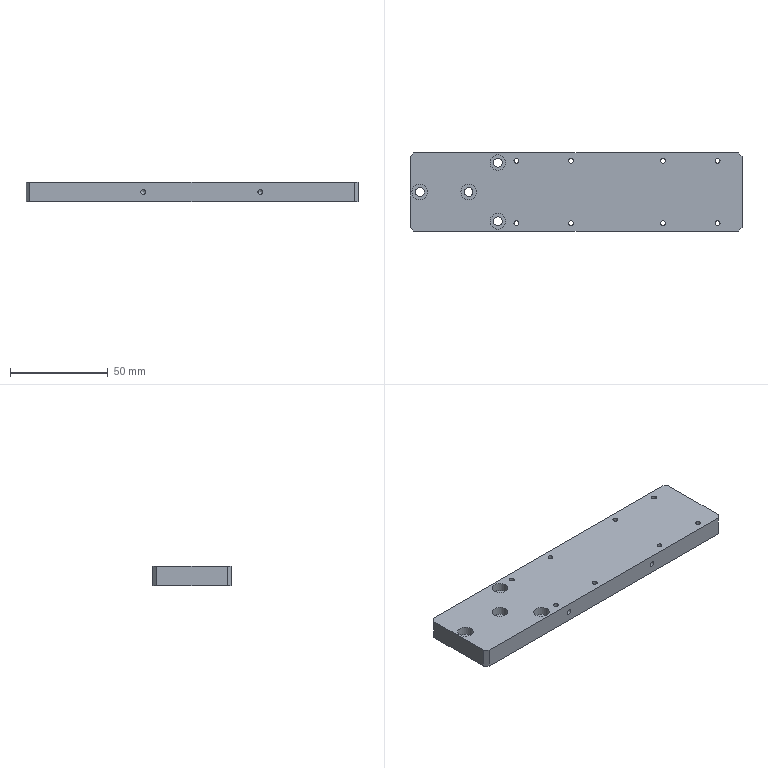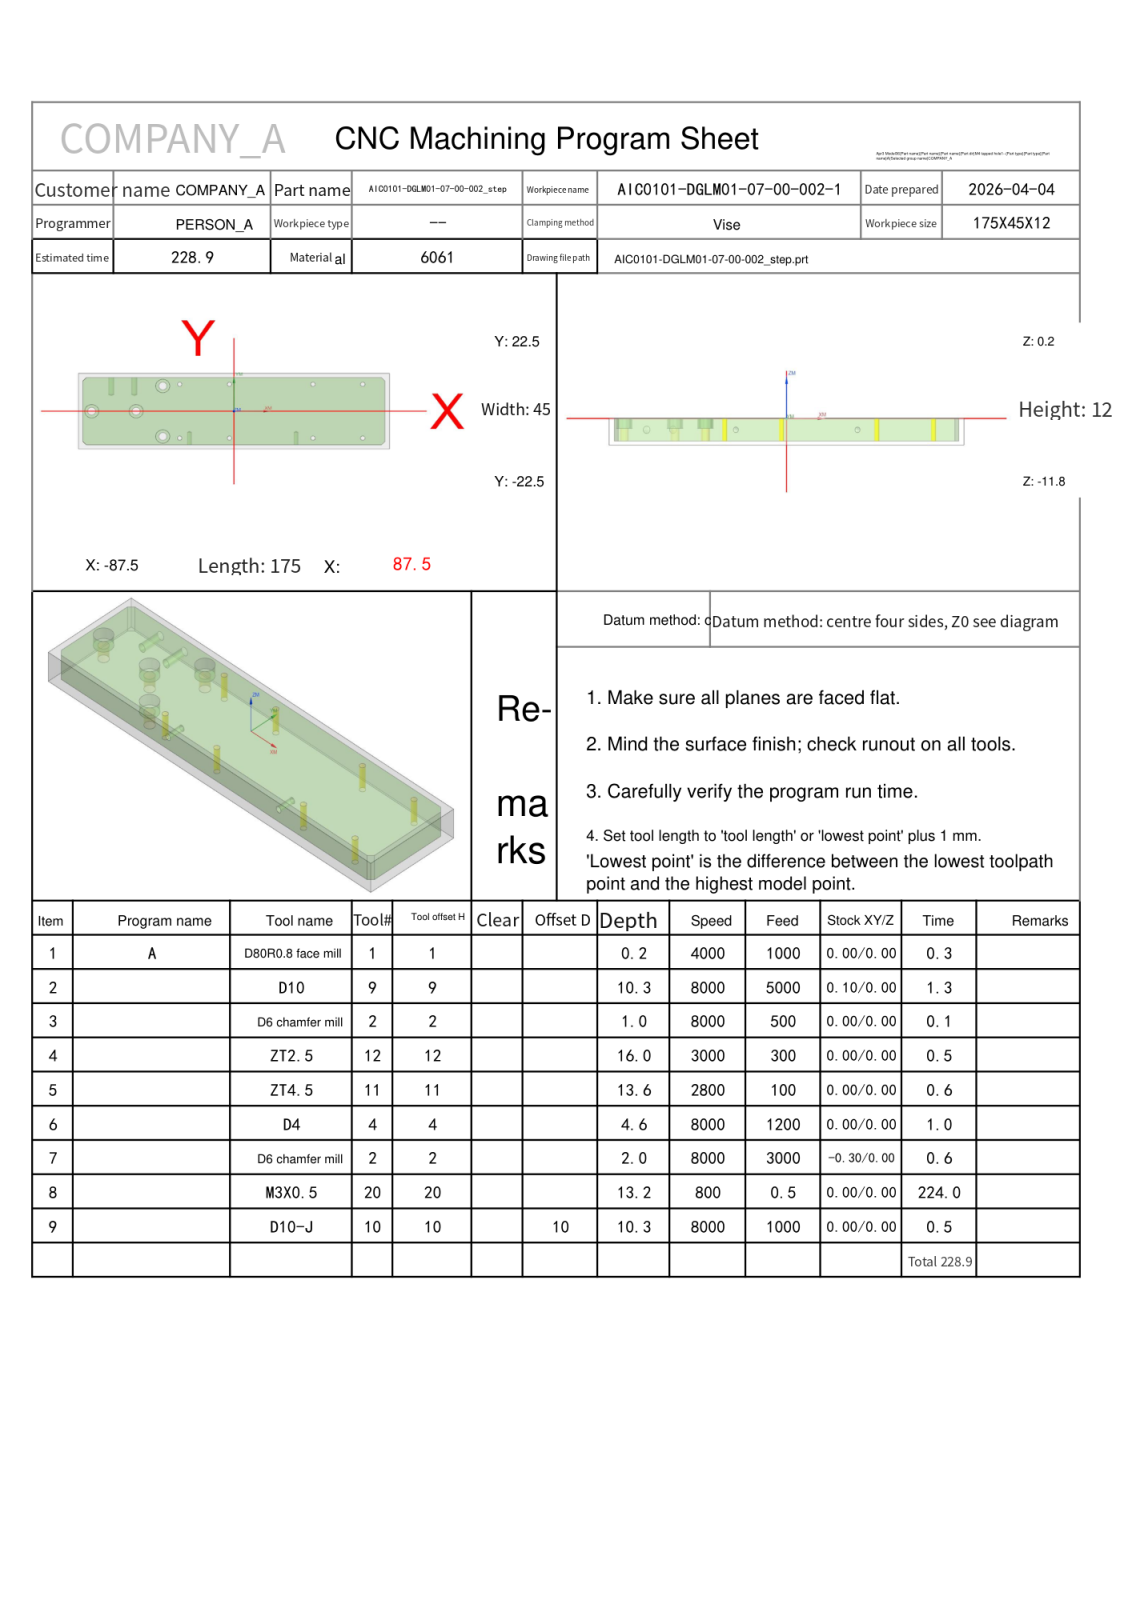NC program | NX | posted by the shop | part box 170 x 40 x 10 mm
Whole program:
%
O0001
(Machine time: 438.58 MIN)
(===Total Tool:8===)
(T1=D80R0.8 face mill D=80.  R=0.8  D-  H01 Z=0.    )
(T9=D10     D=10.  R=0.   D-  H09 Z=-10.1 )
(T2=D6 chamfer mill   D=6.   R=0.   D-  H02 Z=-1.75 )
(T12=ZT2.5  D=2.5  DR_a=118 D-  H12 Z=-15.75)
(T11=ZT4.5  D=4.5  DR_a=118 D-  H11 Z=-13.35)
(T4=D4      D=4.   R=0.   D4  H04 Z=-4.4  )
(T20=M3X0.5 D=2.5  DR_a=180 D-  H20 Z=-13.  )
(T10=D10-J  D=10.  R=0.   D10 H10 Z=-10.1 )
G80 G90 G17 G49 G40
G91 G28 Z0
M01
N1 T01 M06
(D80R0.8 face mill D=80. R=0.8 H=01 ce=0.00 di=0.00)
G00 G90 G54 X-130. Y0.0 M03 S4000
G43 H01 Z20.
M08
Z2.
G01 Z0.0 F1000.
X-125.
X125.
X130.
Z2.
G00 Z20.
G91 G28 Z0.0
M05
M09
G91 G28 Z0.0
M01
N2 T09 M06
(D10  D=10. R=0. H=09 ce=0.10 di=0.00)
G00 G90 G54 X0.0 Y-25.1 M03 S8000
G43 H09 Z20.
M08
Z.5
G01 X-83. Z.36 F5000.
G02 X-86.606 Y-23.606 Z.353 I0.0 J5.1
G01 X-88.606 Y-21.606 Z.348
G02 X-90.1 Y-18. Z.341 I3.606 J3.606
G01 Y18. Z.28
G02 X-88.606 Y21.606 Z.273 I5.1 J0.0
G01 X-86.606 Y23.606 Z.269
G02 X-83. Y25.1 Z.262 I3.606 J-3.606
G01 X83. Z-.019
G02 X86.606 Y23.606 Z-.026 I0.0 J-5.1
G01 X88.606 Y21.606 Z-.031
G02 X90.1 Y18. Z-.037 I-3.606 J-3.606
G01 Y-18. Z-.098
G02 X88.606 Y-21.606 Z-.105 I-5.1 J0.0
G01 X86.606 Y-23.606 Z-.11
G02 X83. Y-25.1 Z-.117 I-3.606 J3.606
G01 X-83. Z-.398
G02 X-86.606 Y-23.606 Z-.404 I0.0 J5.1
G01 X-88.606 Y-21.606 Z-.409
G02 X-90.1 Y-18. Z-.416 I3.606 J3.606
G01 Y18. Z-.477
G02 X-88.606 Y21.606 Z-.484 I5.1 J0.0
G01 X-86.606 Y23.606 Z-.488
G02 X-83. Y25.1 Z-.495 I3.606 J-3.606
G01 X83. Z-.776
G02 X86.606 Y23.606 Z-.783 I0.0 J-5.1
G01 X88.606 Y21.606 Z-.788
G02 X90.1 Y18. Z-.795 I-3.606 J-3.606
G01 Y-18. Z-.855
G02 X88.606 Y-21.606 Z-.862 I-5.1 J0.0
G01 X86.606 Y-23.606 Z-.867
G02 X83. Y-25.1 Z-.874 I-3.606 J3.606
G01 X-83. Z-1.155
G02 X-86.606 Y-23.606 Z-1.162 I0.0 J5.1
G01 X-88.606 Y-21.606 Z-1.166
G02 X-90.1 Y-18. Z-1.173 I3.606 J3.606
G01 Y18. Z-1.234
G02 X-88.606 Y21.606 Z-1.241 I5.1 J0.0
G01 X-86.606 Y23.606 Z-1.246
G02 X-83. Y25.1 Z-1.252 I3.606 J-3.606
G01 X83. Z-1.533
G02 X86.606 Y23.606 Z-1.54 I0.0 J-5.1
G01 X88.606 Y21.606 Z-1.545
G02 X90.1 Y18. Z-1.552 I-3.606 J-3.606
G01 Y-18. Z-1.613
G02 X88.606 Y-21.606 Z-1.619 I-5.1 J0.0
G01 X86.606 Y-23.606 Z-1.624
G02 X83. Y-25.1 Z-1.631 I-3.606 J3.606
G01 X-83. Z-1.912
G02 X-86.606 Y-23.606 Z-1.919 I0.0 J5.1
G01 X-88.606 Y-21.606 Z-1.923
G02 X-90.1 Y-18. Z-1.93 I3.606 J3.606
G01 Y18. Z-1.991
G02 X-88.606 Y21.606 Z-1.998 I5.1 J0.0
G01 X-86.606 Y23.606 Z-2.003
G02 X-83. Y25.1 Z-2.01 I3.606 J-3.606
G01 X83. Z-2.29
G02 X86.606 Y23.606 Z-2.297 I0.0 J-5.1
G01 X88.606 Y21.606 Z-2.302
G02 X90.1 Y18. Z-2.309 I-3.606 J-3.606
G01 Y-18. Z-2.37
G02 X88.606 Y-21.606 Z-2.377 I-5.1 J0.0
G01 X86.606 Y-23.606 Z-2.381
G02 X83. Y-25.1 Z-2.388 I-3.606 J3.606
G01 X-83. Z-2.669
G02 X-86.606 Y-23.606 Z-2.676 I0.0 J5.1
G01 X-88.606 Y-21.606 Z-2.681
G02 X-90.1 Y-18. Z-2.687 I3.606 J3.606
G01 Y18. Z-2.748
G02 X-88.606 Y21.606 Z-2.755 I5.1 J0.0
G01 X-86.606 Y23.606 Z-2.76
G02 X-83. Y25.1 Z-2.767 I3.606 J-3.606
G01 X83. Z-3.048
G02 X86.606 Y23.606 Z-3.054 I0.0 J-5.1
G01 X88.606 Y21.606 Z-3.059
G02 X90.1 Y18. Z-3.066 I-3.606 J-3.606
G01 Y-18. Z-3.127
G02 X88.606 Y-21.606 Z-3.134 I-5.1 J0.0
G01 X86.606 Y-23.606 Z-3.138
G02 X83. Y-25.1 Z-3.145 I-3.606 J3.606
G01 X-83. Z-3.426
G02 X-86.606 Y-23.606 Z-3.433 I0.0 J5.1
G01 X-88.606 Y-21.606 Z-3.438
G02 X-90.1 Y-18. Z-3.445 I3.606 J3.606
G01 Y18. Z-3.505
G02 X-88.606 Y21.606 Z-3.512 I5.1 J0.0
G01 X-86.606 Y23.606 Z-3.517
G02 X-83. Y25.1 Z-3.524 I3.606 J-3.606
G01 X83. Z-3.805
G02 X86.606 Y23.606 Z-3.812 I0.0 J-5.1
G01 X88.606 Y21.606 Z-3.816
G02 X90.1 Y18. Z-3.823 I-3.606 J-3.606
G01 Y-18. Z-3.884
G02 X88.606 Y-21.606 Z-3.891 I-5.1 J0.0
G01 X86.606 Y-23.606 Z-3.896
G02 X83. Y-25.1 Z-3.902 I-3.606 J3.606
G01 X-83. Z-4.183
G02 X-86.606 Y-23.606 Z-4.19 I0.0 J5.1
G01 X-88.606 Y-21.606 Z-4.195
G02 X-90.1 Y-18. Z-4.202 I3.606 J3.606
G01 Y18. Z-4.263
G02 X-88.606 Y21.606 Z-4.269 I5.1 J0.0
G01 X-86.606 Y23.606 Z-4.274
G02 X-83. Y25.1 Z-4.281 I3.606 J-3.606
G01 X83. Z-4.562
G02 X86.606 Y23.606 Z-4.569 I0.0 J-5.1
G01 X88.606 Y21.606 Z-4.573
G02 X90.1 Y18. Z-4.58 I-3.606 J-3.606
G01 Y-18. Z-4.641
G02 X88.606 Y-21.606 Z-4.648 I-5.1 J0.0
G01 X86.606 Y-23.606 Z-4.653
G02 X83. Y-25.1 Z-4.66 I-3.606 J3.606
G01 X-83. Z-4.94
G02 X-86.606 Y-23.606 Z-4.947 I0.0 J5.1
G01 X-88.606 Y-21.606 Z-4.952
G02 X-90.1 Y-18. Z-4.959 I3.606 J3.606
G01 Y18. Z-5.02
G02 X-88.606 Y21.606 Z-5.027 I5.1 J0.0
G01 X-86.606 Y23.606 Z-5.031
G02 X-83. Y25.1 Z-5.038 I3.606 J-3.606
G01 X83. Z-5.319
G02 X86.606 Y23.606 Z-5.326 I0.0 J-5.1
G01 X88.606 Y21.606 Z-5.331
G02 X90.1 Y18. Z-5.337 I-3.606 J-3.606
G01 Y-18. Z-5.398
G02 X88.606 Y-21.606 Z-5.405 I-5.1 J0.0
G01 X86.606 Y-23.606 Z-5.41
G02 X83. Y-25.1 Z-5.417 I-3.606 J3.606
G01 X-83. Z-5.698
G02 X-86.606 Y-23.606 Z-5.704 I0.0 J5.1
G01 X-88.606 Y-21.606 Z-5.709
G02 X-90.1 Y-18. Z-5.716 I3.606 J3.606
G01 Y18. Z-5.777
G02 X-88.606 Y21.606 Z-5.784 I5.1 J0.0
G01 X-86.606 Y23.606 Z-5.788
G02 X-83. Y25.1 Z-5.795 I3.606 J-3.606
G01 X83. Z-6.076
G02 X86.606 Y23.606 Z-6.083 I0.0 J-5.1
G01 X88.606 Y21.606 Z-6.088
G02 X90.1 Y18. Z-6.095 I-3.606 J-3.606
G01 Y-18. Z-6.155
G02 X88.606 Y-21.606 Z-6.162 I-5.1 J0.0
G01 X86.606 Y-23.606 Z-6.167
G02 X83. Y-25.1 Z-6.174 I-3.606 J3.606
G01 X-83. Z-6.455
G02 X-86.606 Y-23.606 Z-6.462 I0.0 J5.1
G01 X-88.606 Y-21.606 Z-6.466
G02 X-90.1 Y-18. Z-6.473 I3.606 J3.606
G01 Y18. Z-6.534
G02 X-88.606 Y21.606 Z-6.541 I5.1 J0.0
G01 X-86.606 Y23.606 Z-6.546
G02 X-83. Y25.1 Z-6.552 I3.606 J-3.606
G01 X83. Z-6.833
G02 X86.606 Y23.606 Z-6.84 I0.0 J-5.1
G01 X88.606 Y21.606 Z-6.845
G02 X90.1 Y18. Z-6.852 I-3.606 J-3.606
G01 Y-18. Z-6.913
G02 X88.606 Y-21.606 Z-6.919 I-5.1 J0.0
G01 X86.606 Y-23.606 Z-6.924
G02 X83. Y-25.1 Z-6.931 I-3.606 J3.606
G01 X-83. Z-7.212
G02 X-86.606 Y-23.606 Z-7.219 I0.0 J5.1
G01 X-88.606 Y-21.606 Z-7.223
G02 X-90.1 Y-18. Z-7.23 I3.606 J3.606
G01 Y18. Z-7.291
G02 X-88.606 Y21.606 Z-7.298 I5.1 J0.0
G01 X-86.606 Y23.606 Z-7.303
G02 X-83. Y25.1 Z-7.31 I3.606 J-3.606
G01 X83. Z-7.59
G02 X86.606 Y23.606 Z-7.597 I0.0 J-5.1
G01 X88.606 Y21.606 Z-7.602
G02 X90.1 Y18. Z-7.609 I-3.606 J-3.606
G01 Y-18. Z-7.67
G02 X88.606 Y-21.606 Z-7.677 I-5.1 J0.0
G01 X86.606 Y-23.606 Z-7.681
G02 X83. Y-25.1 Z-7.688 I-3.606 J3.606
G01 X-83. Z-7.969
G02 X-86.606 Y-23.606 Z-7.976 I0.0 J5.1
G01 X-88.606 Y-21.606 Z-7.981
G02 X-90.1 Y-18. Z-7.987 I3.606 J3.606
G01 Y18. Z-8.048
G02 X-88.606 Y21.606 Z-8.055 I5.1 J0.0
G01 X-86.606 Y23.606 Z-8.06
G02 X-83. Y25.1 Z-8.067 I3.606 J-3.606
G01 X83. Z-8.348
G02 X86.606 Y23.606 Z-8.354 I0.0 J-5.1
G01 X88.606 Y21.606 Z-8.359
G02 X90.1 Y18. Z-8.366 I-3.606 J-3.606
G01 Y-18. Z-8.427
G02 X88.606 Y-21.606 Z-8.434 I-5.1 J0.0
G01 X86.606 Y-23.606 Z-8.438
G02 X83. Y-25.1 Z-8.445 I-3.606 J3.606
G01 X-83. Z-8.726
G02 X-86.606 Y-23.606 Z-8.733 I0.0 J5.1
G01 X-88.606 Y-21.606 Z-8.738
G02 X-90.1 Y-18. Z-8.745 I3.606 J3.606
G01 Y18. Z-8.805
G02 X-88.606 Y21.606 Z-8.812 I5.1 J0.0
G01 X-86.606 Y23.606 Z-8.817
G02 X-83. Y25.1 Z-8.824 I3.606 J-3.606
G01 X83. Z-9.105
G02 X86.606 Y23.606 Z-9.112 I0.0 J-5.1
G01 X88.606 Y21.606 Z-9.116
G02 X90.1 Y18. Z-9.123 I-3.606 J-3.606
G01 Y-18. Z-9.184
G02 X88.606 Y-21.606 Z-9.191 I-5.1 J0.0
G01 X86.606 Y-23.606 Z-9.196
G02 X83. Y-25.1 Z-9.202 I-3.606 J3.606
G01 X-83. Z-9.483
G02 X-86.606 Y-23.606 Z-9.49 I0.0 J5.1
G01 X-88.606 Y-21.606 Z-9.495
G02 X-90.1 Y-18. Z-9.502 I3.606 J3.606
G01 Y18. Z-9.563
G02 X-88.606 Y21.606 Z-9.569 I5.1 J0.0
G01 X-86.606 Y23.606 Z-9.574
G02 X-83. Y25.1 Z-9.581 I3.606 J-3.606
G01 X83. Z-9.862
G02 X86.606 Y23.606 Z-9.869 I0.0 J-5.1
G01 X88.606 Y21.606 Z-9.873
G02 X90.1 Y18. Z-9.88 I-3.606 J-3.606
G01 Y-18. Z-9.941
G02 X88.606 Y-21.606 Z-9.948 I-5.1 J0.0
G01 X86.606 Y-23.606 Z-9.953
G02 X83. Y-25.1 Z-9.96 I-3.606 J3.606
G01 X0.0 Z-10.1
X-83.
G02 X-86.606 Y-23.606 I0.0 J5.1
G01 X-88.606 Y-21.606
G02 X-90.1 Y-18. I3.606 J3.606
G01 Y18.
G02 X-88.606 Y21.606 I5.1 J0.0
G01 X-86.606 Y23.606
G02 X-83. Y25.1 I3.606 J-3.606
G01 X83.
G02 X86.606 Y23.606 I0.0 J-5.1
G01 X88.606 Y21.606
G02 X90.1 Y18. I-3.606 J-3.606
G01 Y-18.
G02 X88.606 Y-21.606 I-5.1 J0.0
G01 X86.606 Y-23.606
G02 X83. Y-25.1 I-3.606 J3.606
G01 X0.0
X-.5
Z-9.1
G00 Z20.
G91 G28 Z0.0
M05
M09
G91 G28 Z0.0
M01
N3 T02 M06
(D6 chamfer mill D=6. R=0. H=02 ce=0.00 di=0.00)
G00 G90 G54 X-80. Y0.0 M03 S8000
G43 H02 Z20.
M08
G98 G81 X-80. Y0.0 Z-.8 R1. F500.
X-55.
X-40. Y-15.
X-30.5 Y-16.
X-40. Y15.
X-30.5 Y16.
X-2.5
Y-16.
X44.5
X72.5
Y16.
X44.5
G80
G00 Z20.
G91 G28 Z0.0
M05
M09
G91 G28 Z0.0
M01
N4 T12 M06
(ZT2.5 D=2.5 DR_a=118 H=12)
G00 G90 G54 X44.5 Y-16. M03 S3000
G43 H12 Z20.
M08
G98 G83 X44.5 Y-16. Z-15.751 R1. F300. Q2.
X72.5
Y16.
X44.5
X-2.5
X-30.5
Y-16.
X-2.5
G80
G00 Z20.
G91 G28 Z0.0
M05
M09
G91 G28 Z0.0
M01
N5 T11 M06
(ZT4.5 D=4.5 DR_a=118 H=11)
G00 G90 G54 X-40. Y-15. M03 S2800
G43 H11 Z20.
M08
G98 G83 X-40. Y-15. Z-13.352 R1. F100. Q2.
Y15.
X-55. Y0.0
X-80.
G80
G00 Z20.
G91 G28 Z0.0
M05
M09
G91 G28 Z0.0
M01
N6 T04 M06
(D4  D=4. R=0. H=04 ce=0.10 di=0.00)
G00 G90 G54 X-40. Y-15. M03 S8000
G43 H04 Z20.
M08
Z.5
G03 X-39.05 Y-15.95 I.95 J0.0 F1200.
X-38.1 Y-15. I0.0 J.95
X-38.1 Y-15. Z.2 I-1.9 J0.0
X-38.1 Y-15. Z-.1 I-1.9 J0.0
X-38.1 Y-15. Z-.4 I-1.9 J0.0
X-38.1 Y-15. Z-.7 I-1.9 J0.0
X-38.1 Y-15. Z-1. I-1.9 J0.0
X-38.1 Y-15. Z-1.3 I-1.9 J0.0
X-38.1 Y-15. Z-1.6 I-1.9 J0.0
X-38.1 Y-15. Z-1.9 I-1.9 J0.0
X-38.1 Y-15. Z-2.2 I-1.9 J0.0
X-38.1 Y-15. Z-2.5 I-1.9 J0.0
X-38.1 Y-15. Z-2.8 I-1.9 J0.0
X-38.1 Y-15. Z-3.1 I-1.9 J0.0
X-38.1 Y-15. Z-3.4 I-1.9 J0.0
X-38.1 Y-15. Z-3.7 I-1.9 J0.0
X-38.1 Y-15. Z-4. I-1.9 J0.0
X-38.1 Y-15. Z-4.3 I-1.9 J0.0
X-40.95 Y-13.355 Z-4.4 I-1.9 J0.0
X-41.9 Y-15. I.95 J-1.645
X-40. Y-16.9 I1.9 J0.0
X-38.1 Y-15. I0.0 J1.9
X-40. Y-13.1 I-1.9 J0.0
X-40.95 Y-13.355 I0.0 J-1.9
X-41.425 Y-14.177 I.475 J-.823
X-40.475 Y-15.127 I.95 J0.0
X-40. Y-15. I0.0 J.95
G00 Z20.
Y15.
Z.5
G03 X-39.05 Y14.05 I.95 J0.0
X-38.1 Y15. I0.0 J.95
X-38.1 Y15. Z.2 I-1.9 J0.0
X-38.1 Y15. Z-.1 I-1.9 J0.0
X-38.1 Y15. Z-.4 I-1.9 J0.0
X-38.1 Y15. Z-.7 I-1.9 J0.0
X-38.1 Y15. Z-1. I-1.9 J0.0
X-38.1 Y15. Z-1.3 I-1.9 J0.0
X-38.1 Y15. Z-1.6 I-1.9 J0.0
X-38.1 Y15. Z-1.9 I-1.9 J0.0
X-38.1 Y15. Z-2.2 I-1.9 J0.0
X-38.1 Y15. Z-2.5 I-1.9 J0.0
X-38.1 Y15. Z-2.8 I-1.9 J0.0
X-38.1 Y15. Z-3.1 I-1.9 J0.0
X-38.1 Y15. Z-3.4 I-1.9 J0.0
X-38.1 Y15. Z-3.7 I-1.9 J0.0
X-38.1 Y15. Z-4. I-1.9 J0.0
X-38.1 Y15. Z-4.3 I-1.9 J0.0
X-40.95 Y16.645 Z-4.4 I-1.9 J0.0
X-41.9 Y15. I.95 J-1.645
X-40. Y13.1 I1.9 J0.0
X-38.1 Y15. I0.0 J1.9
X-40. Y16.9 I-1.9 J0.0
X-40.95 Y16.645 I0.0 J-1.9
X-41.425 Y15.823 I.475 J-.823
X-40.475 Y14.873 I.95 J0.0
X-40. Y15. I0.0 J.95
G00 Z20.
X-55. Y0.0
Z.5
G03 X-54.05 Y-.95 I.95 J0.0
X-53.1 Y0.0 I0.0 J.95
X-53.1 Y0.0 Z.2 I-1.9 J0.0
X-53.1 Y0.0 Z-.1 I-1.9 J0.0
X-53.1 Y0.0 Z-.4 I-1.9 J0.0
X-53.1 Y0.0 Z-.7 I-1.9 J0.0
X-53.1 Y0.0 Z-1. I-1.9 J0.0
X-53.1 Y0.0 Z-1.3 I-1.9 J0.0
X-53.1 Y0.0 Z-1.6 I-1.9 J0.0
X-53.1 Y0.0 Z-1.9 I-1.9 J0.0
X-53.1 Y0.0 Z-2.2 I-1.9 J0.0
X-53.1 Y0.0 Z-2.5 I-1.9 J0.0
X-53.1 Y0.0 Z-2.8 I-1.9 J0.0
X-53.1 Y0.0 Z-3.1 I-1.9 J0.0
X-53.1 Y0.0 Z-3.4 I-1.9 J0.0
X-53.1 Y0.0 Z-3.7 I-1.9 J0.0
X-53.1 Y0.0 Z-4. I-1.9 J0.0
X-53.1 Y0.0 Z-4.3 I-1.9 J0.0
X-55.95 Y1.645 Z-4.4 I-1.9 J0.0
X-56.9 Y0.0 I.95 J-1.645
X-55. Y-1.9 I1.9 J0.0
X-53.1 Y0.0 I0.0 J1.9
X-55. Y1.9 I-1.9 J0.0
X-55.95 Y1.645 I0.0 J-1.9
X-56.425 Y.823 I.475 J-.823
X-55.475 Y-.127 I.95 J0.0
X-55. Y0.0 I0.0 J.95
G00 Z20.
X-80.
Z.5
G03 X-79.05 Y-.95 I.95 J0.0
X-78.1 Y0.0 I0.0 J.95
X-78.1 Y0.0 Z.2 I-1.9 J0.0
X-78.1 Y0.0 Z-.1 I-1.9 J0.0
X-78.1 Y0.0 Z-.4 I-1.9 J0.0
X-78.1 Y0.0 Z-.7 I-1.9 J0.0
X-78.1 Y0.0 Z-1. I-1.9 J0.0
X-78.1 Y0.0 Z-1.3 I-1.9 J0.0
X-78.1 Y0.0 Z-1.6 I-1.9 J0.0
X-78.1 Y0.0 Z-1.9 I-1.9 J0.0
X-78.1 Y0.0 Z-2.2 I-1.9 J0.0
X-78.1 Y0.0 Z-2.5 I-1.9 J0.0
X-78.1 Y0.0 Z-2.8 I-1.9 J0.0
X-78.1 Y0.0 Z-3.1 I-1.9 J0.0
X-78.1 Y0.0 Z-3.4 I-1.9 J0.0
X-78.1 Y0.0 Z-3.7 I-1.9 J0.0
X-78.1 Y0.0 Z-4. I-1.9 J0.0
X-78.1 Y0.0 Z-4.3 I-1.9 J0.0
X-80.95 Y1.645 Z-4.4 I-1.9 J0.0
X-81.9 Y0.0 I.95 J-1.645
X-80. Y-1.9 I1.9 J0.0
X-78.1 Y0.0 I0.0 J1.9
X-80. Y1.9 I-1.9 J0.0
X-80.95 Y1.645 I0.0 J-1.9
X-81.425 Y.823 I.475 J-.823
X-80.475 Y-.127 I.95 J0.0
X-80. Y0.0 I0.0 J.95
G00 Z20.
G00 G90 X-40. Y-15. M03 S8000
Z20.
Z.5
G41 D04
G01 X-39.96 Y-15.196 F500.
G03 X-38.99 Y-15.99 I.97 J.196
X-38. Y-15. I0.0 J.99
X-38.016 Y-15.251 Z-4.4 I-2. J0.0
X-38. Y-15. I-1.984 J.251
X-40. Y-13. I-2. J0.0
X-42. Y-15. I0.0 J-2.
X-40. Y-17. I2. J0.0
X-38.016 Y-15.251 I0.0 J2.
G01 X-38.008 Y-15.127
G03 X-38.998 Y-14.137 I-.99 J0.0
X-39.936 Y-14.81 I0.0 J-.99
G01 G40 X-40. Y-15.
G00 Z20.
Y15.
Z.5
G41 D04
G01 X-39.96 Y14.804
G03 X-38.99 Y14.01 I.97 J.196
X-38. Y15. I0.0 J.99
X-38.016 Y14.749 Z-4.4 I-2. J0.0
X-38. Y15. I-1.984 J.251
X-40. Y17. I-2. J0.0
X-42. Y15. I0.0 J-2.
X-40. Y13. I2. J0.0
X-38.016 Y14.749 I0.0 J2.
G01 X-38.008 Y14.873
G03 X-38.998 Y15.863 I-.99 J0.0
X-39.936 Y15.19 I0.0 J-.99
G01 G40 X-40. Y15.
G00 Z20.
X-55. Y0.0
Z.5
G41 D04
G01 X-54.96 Y-.196
G03 X-53.99 Y-.99 I.97 J.196
X-53. Y0.0 I0.0 J.99
X-53.016 Y-.251 Z-4.4 I-2. J0.0
X-53. Y0.0 I-1.984 J.251
X-55. Y2. I-2. J0.0
X-57. Y0.0 I0.0 J-2.
X-55. Y-2. I2. J0.0
X-53.016 Y-.251 I0.0 J2.
G01 X-53.008 Y-.127
G03 X-53.998 Y.863 I-.99 J0.0
X-54.936 Y.19 I0.0 J-.99
G01 G40 X-55. Y0.0
G00 Z20.
X-80.
Z.5
G41 D04
G01 X-79.96 Y-.196
G03 X-78.99 Y-.99 I.97 J.196
X-78. Y0.0 I0.0 J.99
X-78.016 Y-.251 Z-4.4 I-2. J0.0
X-78. Y0.0 I-1.984 J.251
X-80. Y2. I-2. J0.0
X-82. Y0.0 I0.0 J-2.
X-80. Y-2. I2. J0.0
X-78.016 Y-.251 I0.0 J2.
G01 X-78.008 Y-.127
G03 X-78.998 Y.863 I-.99 J0.0
X-79.936 Y.19 I0.0 J-.99
G01 G40 X-80. Y0.0
G00 Z20.
G91 G28 Z0.0
M05
M09
G91 G28 Z0.0
M01
N7 T02 M06
(D6 chamfer mill D=6. R=0. H=02 ce=0.00 di=0.00)
G00 G90 G54 X-.25 Y22.128 M03 S8000
G43 H02 Z20.
M08
Z2.099
G01 Z-1.5 F3000.
G03 X-.33 Y21.828 I.52 J-.3
X-.03 Y21.308 I.6 J0.0
G01 X0.0 Y21.3
X83.
X83.254 Y21.275
X83.497 Y21.201
X83.722 Y21.081
X83.919 Y20.919
X85.919 Y18.919
X86.081 Y18.722
X86.201 Y18.497
X86.275 Y18.254
X86.3 Y18.
Y-18.
X86.275 Y-18.254
X86.201 Y-18.497
X86.081 Y-18.722
X85.919 Y-18.919
X83.919 Y-20.919
X83.722 Y-21.081
X83.497 Y-21.201
X83.254 Y-21.275
X83. Y-21.3
X-83.
X-83.254 Y-21.275
X-83.497 Y-21.201
X-83.722 Y-21.081
X-83.919 Y-20.919
X-85.919 Y-18.919
X-86.081 Y-18.722
X-86.201 Y-18.497
X-86.275 Y-18.254
X-86.3 Y-18.
Y18.
X-86.275 Y18.254
X-86.201 Y18.497
X-86.081 Y18.722
X-85.919 Y18.919
X-83.919 Y20.919
X-83.722 Y21.081
X-83.497 Y21.201
X-83.254 Y21.275
X-83. Y21.3
X0.0
X.03 Y21.308
G03 X.33 Y21.828 I-.3 J.52
X.25 Y22.128 I-.6 J0.0
G01 Z2.099
G00 Z20.
G00 G90 X44.5 Y-16. M03 S8000
Z20.
G98 G81 X44.5 Y-16. Z-1.75 R3. F500.
X72.5
Y16.
X44.5
X-2.5
X-30.5
Y-16.
X-2.5
G80
G00 Z20.
G00 G90 X-43.212 Y-15.747 M03 S8000
Z20.
Z2.5
G01 X-43.16 Y-15.962 Z2.42 F500.
X-43.024 Y-16.328 Z2.278
X-42.847 Y-16.675 Z2.136
X-42.629 Y-16.999 Z1.994
X-42.375 Y-17.295 Z1.852
X-42.088 Y-17.559 Z1.71
X-41.772 Y-17.788 Z1.568
X-41.528 Y-17.928 Z1.465
X-41.172 Y-18.088 Z1.323
X-40.8 Y-18.205 Z1.181
X-40.416 Y-18.277 Z1.039
X-40.027 Y-18.303 Z.897
X-39.638 Y-18.283 Z.755
X-39.253 Y-18.217 Z.613
X-38.879 Y-18.107 Z.471
X-38.52 Y-17.953 Z.329
X-38.182 Y-17.758 Z.187
X-37.87 Y-17.524 Z.045
X-37.587 Y-17.256 Z-.097
X-37.338 Y-16.955 Z-.239
X-37.126 Y-16.628 Z-.381
X-36.954 Y-16.278 Z-.523
X-36.825 Y-15.91 Z-.665
X-36.74 Y-15.529 Z-.807
X-36.7 Y-15.141 Z-.949
Y-15. Z-1.
G03 X-40. Y-11.7 I-3.3 J0.0
X-43.3 Y-15. I0.0 J-3.3
X-40. Y-18.3 I3.3 J0.0
X-36.7 Y-15. I0.0 J3.3
X-36.738 Y-14.502 I-3.3 J0.0
G01 Z1.5
G00 Z20.
X-43.212 Y14.253
Z2.5
G01 X-43.16 Y14.038 Z2.42
X-43.024 Y13.672 Z2.278
X-42.847 Y13.325 Z2.136
X-42.629 Y13.001 Z1.994
X-42.375 Y12.705 Z1.852
X-42.088 Y12.441 Z1.71
X-41.772 Y12.212 Z1.568
X-41.528 Y12.072 Z1.465
X-41.172 Y11.912 Z1.323
X-40.8 Y11.795 Z1.181
X-40.416 Y11.723 Z1.039
X-40.027 Y11.697 Z.897
X-39.638 Y11.717 Z.755
X-39.253 Y11.783 Z.613
X-38.879 Y11.893 Z.471
X-38.52 Y12.047 Z.329
X-38.182 Y12.242 Z.187
X-37.87 Y12.476 Z.045
X-37.587 Y12.744 Z-.097
X-37.338 Y13.045 Z-.239
X-37.126 Y13.372 Z-.381
X-36.954 Y13.722 Z-.523
X-36.825 Y14.09 Z-.665
X-36.74 Y14.471 Z-.807
X-36.7 Y14.859 Z-.949
Y15. Z-1.
G03 X-40. Y18.3 I-3.3 J0.0
X-43.3 Y15. I0.0 J-3.3
X-40. Y11.7 I3.3 J0.0
X-36.7 Y15. I0.0 J3.3
X-36.738 Y15.498 I-3.3 J0.0
G01 Z1.5
G00 Z20.
X-58.212 Y-.747
Z2.5
G01 X-58.16 Y-.962 Z2.42
X-58.024 Y-1.328 Z2.278
X-57.847 Y-1.675 Z2.136
X-57.629 Y-1.999 Z1.994
X-57.375 Y-2.295 Z1.852
X-57.088 Y-2.559 Z1.71
X-56.772 Y-2.788 Z1.568
X-56.528 Y-2.928 Z1.465
X-56.172 Y-3.088 Z1.323
X-55.8 Y-3.205 Z1.181
X-55.416 Y-3.277 Z1.039
X-55.027 Y-3.303 Z.897
X-54.638 Y-3.283 Z.755
X-54.253 Y-3.217 Z.613
X-53.879 Y-3.107 Z.471
X-53.52 Y-2.953 Z.329
X-53.182 Y-2.758 Z.187
X-52.87 Y-2.524 Z.045
X-52.587 Y-2.256 Z-.097
X-52.338 Y-1.955 Z-.239
X-52.126 Y-1.628 Z-.381
X-51.954 Y-1.278 Z-.523
X-51.825 Y-.91 Z-.665
X-51.74 Y-.529 Z-.807
X-51.7 Y-.141 Z-.949
Y0.0 Z-1.
G03 X-55. Y3.3 I-3.3 J0.0
X-58.3 Y0.0 I0.0 J-3.3
X-55. Y-3.3 I3.3 J0.0
X-51.7 Y0.0 I0.0 J3.3
X-51.738 Y.498 I-3.3 J0.0
G01 Z1.5
G00 Z20.
X-83.212 Y-.747
Z2.5
G01 X-83.16 Y-.962 Z2.42
X-83.024 Y-1.328 Z2.278
X-82.847 Y-1.675 Z2.136
X-82.629 Y-1.999 Z1.994
X-82.375 Y-2.295 Z1.852
X-82.088 Y-2.559 Z1.71
X-81.772 Y-2.788 Z1.568
X-81.528 Y-2.928 Z1.465
X-81.172 Y-3.088 Z1.323
X-80.8 Y-3.205 Z1.181
X-80.416 Y-3.277 Z1.039
X-80.027 Y-3.303 Z.897
X-79.638 Y-3.283 Z.755
X-79.253 Y-3.217 Z.613
X-78.879 Y-3.107 Z.471
X-78.52 Y-2.953 Z.329
X-78.182 Y-2.758 Z.187
X-77.87 Y-2.524 Z.045
X-77.587 Y-2.256 Z-.097
X-77.338 Y-1.955 Z-.239
X-77.126 Y-1.628 Z-.381
X-76.954 Y-1.278 Z-.523
X-76.825 Y-.91 Z-.665
X-76.74 Y-.529 Z-.807
X-76.7 Y-.141 Z-.949
Y0.0 Z-1.
G03 X-80. Y3.3 I-3.3 J0.0
X-83.3 Y0.0 I0.0 J-3.3
X-80. Y-3.3 I3.3 J0.0
X-76.7 Y0.0 I0.0 J3.3
X-76.738 Y.498 I-3.3 J0.0
G01 Z1.5
G00 Z20.
G91 G28 Z0.0
M05
M09
G91 G28 Z0.0
M01
N8 T20 M06
(M3X0.5 D=2.5 DR_a=180 H=20)
G00 G90 G54 X44.5 Y-16. M03 S800
G43 H20 Z20.
M08
G95
G98 G84 X44.5 Y-16. Z-13. R1. F.5 Q5.
X72.5
Y16.
X44.5
X-2.5
X-30.5
Y-16.
X-2.5
G80
G94
G00 Z20.
G91 G28 Z0.0
M05
M09
G91 G28 Z0.0
M01
N9 T10 M06
(D10-J  D=10. R=0. H=10 ce=0.00 di=0.00)
G00 G90 G54 X84.013 Y-26.116 M03 S8000
G43 H10 Z20.
M08
Z-9.6
G01 Z-10.1 F1000.
G41 D10
X83.997 Y-25.917
G03 X83. Y-25. I-.997 J-.083
G01 X-83.
G02 X-86.536 Y-23.536 I0.0 J5.
G01 X-88.536 Y-21.536
G02 X-90. Y-18. I3.536 J3.536
G01 Y18.
G02 X-88.536 Y21.536 I5. J0.0
G01 X-86.536 Y23.536
G02 X-83. Y25. I3.536 J-3.536
G01 X83.
G02 X86.536 Y23.536 I0.0 J-5.
G01 X88.536 Y21.536
G02 X90. Y18. I-3.536 J-3.536
G01 Y-18.
G02 X88.536 Y-21.536 I-5. J0.0
G01 X86.536 Y-23.536
G02 X83. Y-25. I-3.536 J3.536
G01 X82.5
G03 X81.5 Y-26. I0.0 J-1.
G01 G40 Y-26.2
Z-9.6
G00 Z20.
M05
M09
G91 G28 Z0.0
G91 G28 Y0.0
M30
%